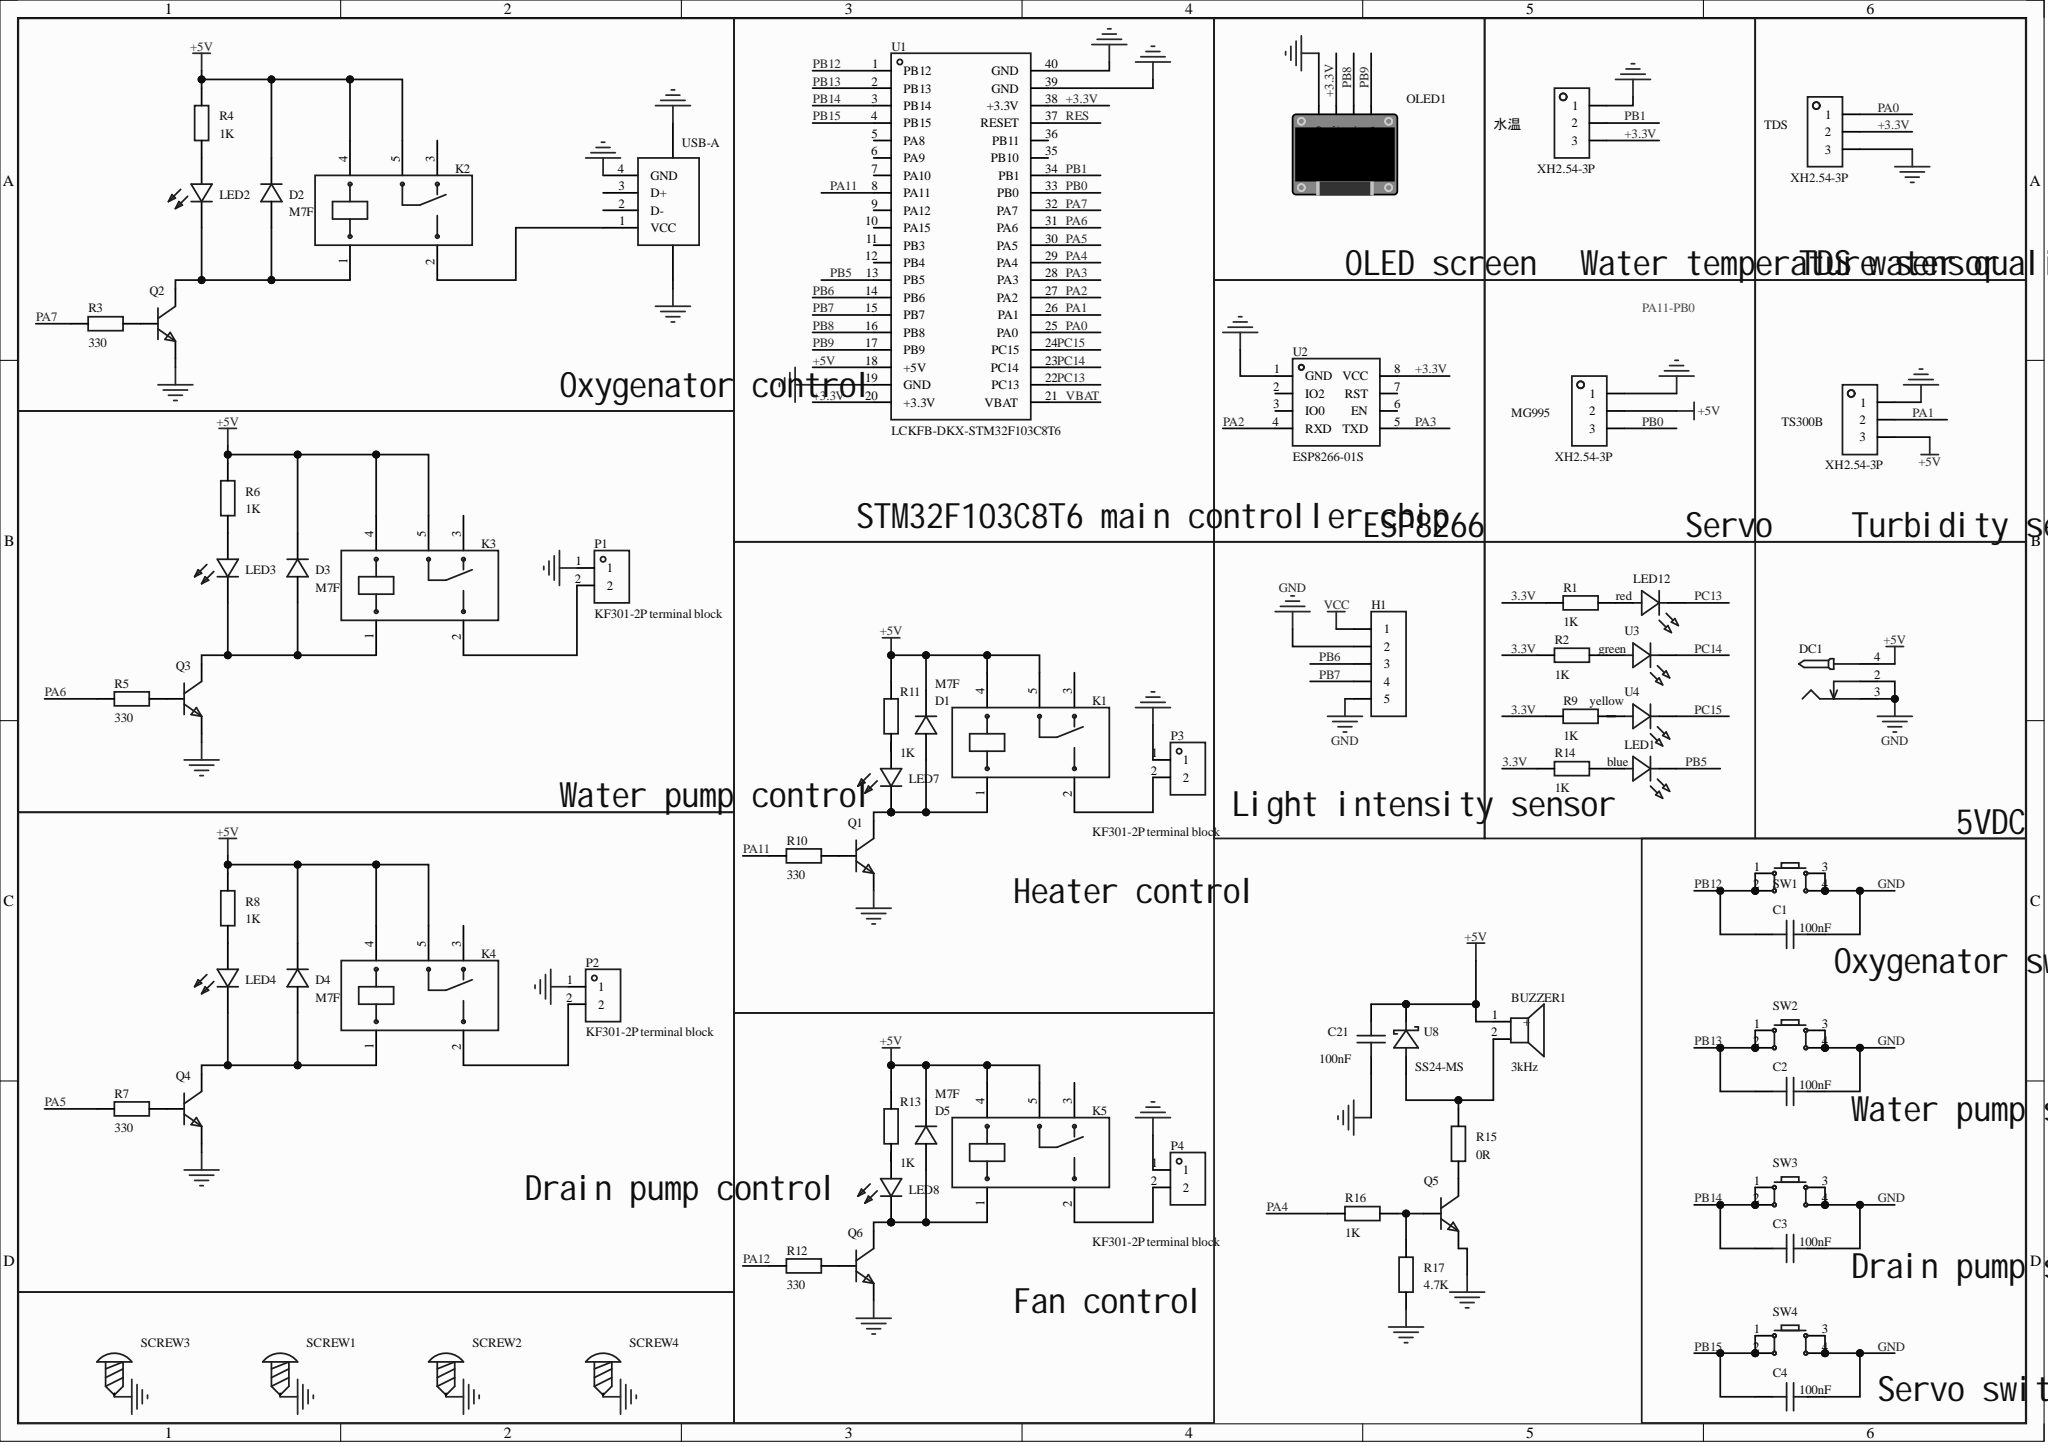Circuit board | Altium Designer | 71 parts | 53 nets
Bill of materials:
Comment,Description,Designator,Footprint,LibRef,Quantity
"3kHz","Drive method: Active (built-in driver circuit); Construction type: Electromagnetic; Rated voltage: -; Frequency: 3kHz; Sound pressure (SPL): 85dB;","BUZZER1","BUZ-TH_BD9.6-P5.00-D0.7-FD","HNB09A05","1"
"100nF","Capacitance: 100nF; Tolerance: ±10%; Rated voltage: 6.3V; Dielectric (temp. coefficient): X7R;, [NoValue]","C1, C2, C3, C4, C21","C0603","CC0603KRX7R5BB104, CAP_0603","5"
"M7F","Forward voltage drop (Vf): 1.1V@1A; DC reverse withstand voltage (Vr): 1kV; Rectifier current: 1A;","D1, D2, D3, D4, D5","SMAF_L3.5-W2.6-LS4.7-RD","M7F_C22368801","5"
"","","DC1","DC-2.0","DC-005_2.0","1"
"","","H1","HDR-TH_5P-P2.54-V-F","HDR-F_2.54_1x5P","1"
"SRD-DC5V-SL-C","Contact form: -;","K1, K2, K3, K4, K5","RELAY-TH_SRD-DCXXV-SL-C","SRD-DC5V-SL-C","5"
"blue","Lamp holder type: 5mm round lamp holder; Emitting color: Blue; Forward voltage drop (Vf): 3.4V; Power: 70mW; Forward current: 20mA; Wavelength: 460nm~470nm; Diode configuration: -; Lens color: Blue lens; Color temperature: -; Luminous intensity: 3cd; Viewing angle: 25°; Tape and reel: -; Operating temperature: -20℃~+85℃;","LED1","LED-TH_BD5.9-P2.54-RD_BLUE","XL-502UBD","1"
"MS-PTV1608NWAF-B02","","LED2, LED3, LED4, LED7, LED8","LED0603-RD","MS-PTV1608NWAF-B02","5"
"red","Lamp holder type: 5mm round lamp holder; Emitting color: Red; Forward voltage drop (Vf): 2.4V; Power: 70mW; Forward current: 20mA; Wavelength: 615nm~625nm; Diode configuration: -; Lens color: Red lens; Color temperature: -; Luminous intensity: 300mcd; Viewing angle: 35°; Tape and reel: -; Operating temperature: -25℃~+85℃;","LED12","LED-TH_BD5.9-P2.54-RD_RED","XL-502SURD","1"
"","","MG995, TDS, TS300B, 水温","XH2.54-3P","弯针座3P","4"
"","","OLED1","0.96OLED_4P","0.96OLED模块_4P","1"
"KF301-2P terminal block","","P1, P2, P3, P4","CONN-TH_XY301V-A-5.0-2P","KF301-2P接线端子","4"
"","","Q1, Q2, Q3, Q4, Q5, Q6","S8050_SOT-23","S8050_SOT_NPN","6"
"1K","","R1, R2, R4, R6, R8, R9, R11, R13, R14, R16","R0603","Res_0603","10"
"330","","R3, R5, R7, R10, R12","R0603","Res_0603","5"
"0R","","R15","R0603","Res_0603","1"
"4.7K","","R17","R0603","Res_0603","1"
"","","SCREW1, SCREW2, SCREW3, SCREW4","M3螺丝","M3螺丝","4"
"","","SW1, SW2, SW3, SW4","SW-SMD_4P-L6.0-W6.0-P4.50-LS9.0-2","Key_SMD_6x6x6.5","4"
"LCKFB-DKX-STM32F103C8T6","","U1","CONN-TH_L53.3-W22.9_STM32F103C8T6-CARD","LCKFB-DKX-STM32F103C8T6","1"
"ESP8266-01S","","U2","WIFIM-TH_ESP8266-01S","ESP8266-01S","1"
"green","Lamp holder type: 5mm round lamp holder; Emitting color: Emerald green; Forward voltage drop (Vf): 3V; Power: 70mW; Forward current: 20mA; Wavelength: 520nm~530nm; Diode configuration: -; Lens color: Green lens; Color temperature: -; Luminous intensity: 12cd; Viewing angle: 25°; Tape and reel: -; Operating temperature: -25℃~+85℃;","U3","LED-TH_BD5.9-P2.54-RD_GREEN","XL-502UGD","1"
"yellow","Lamp holder type: 5mm round lamp holder; Emitting color: Yellow; Forward voltage drop (Vf): 2.2V; Power: 50mW; Forward current: 20mA; Wavelength: 585nm~595nm; Diode configuration: -; Lens color: Yellow lens; Color temperature: -; Luminous intensity: 1cd; Viewing angle: 25°; Tape and reel: -; Operating temperature: -20℃~+85℃;","U4","LED-TH_BD5.9-P2.54-RD_YELLOW","XL-502UYD","1"
"SS24-MS","Diode configuration: -; Forward voltage drop (Vf): 550mV@2A; DC reverse withstand voltage (Vr): 40V; Rectifier current: 2A;","U8","SMA_L4.3-W2.6-LS5.1-RD","SS24-MS","1"
"USB-AF","","USB-A","USB-A-TH_USB-302-T","USB-AF","1"
Netlist (Protel format):
[
BUZZER1
BUZ-TH_BD9.6-P5.00-D0.7-FD
3kHz



]
[
C1
C0603
100nF



]
[
C2
C0603
100nF



]
[
C3
C0603
100nF



]
[
C4
C0603
100nF



]
[
C21
C0603
100nF



]
[
D1
SMAF_L3.5-W2.6-LS4.7-RD
M7F



]
[
D2
SMAF_L3.5-W2.6-LS4.7-RD
M7F



]
[
D3
SMAF_L3.5-W2.6-LS4.7-RD
M7F



]
[
D4
SMAF_L3.5-W2.6-LS4.7-RD
M7F



]
[
D5
SMAF_L3.5-W2.6-LS4.7-RD
M7F



]
[
DC1
DC-2.0




]
[
H1
HDR-TH_5P-P2.54-V-F




]
[
K1
RELAY-TH_SRD-DCXXV-SL-C
SRD-DC5V-SL-C



]
[
K2
RELAY-TH_SRD-DCXXV-SL-C
SRD-DC5V-SL-C



]
[
K3
RELAY-TH_SRD-DCXXV-SL-C
SRD-DC5V-SL-C



]
[
K4
RELAY-TH_SRD-DCXXV-SL-C
SRD-DC5V-SL-C



]
[
K5
RELAY-TH_SRD-DCXXV-SL-C
SRD-DC5V-SL-C



]
[
LED1
LED-TH_BD5.9-P2.54-RD_BLUE
blue



]
[
LED2
LED0603-RD
MS-PTV1608NWAF-B02



]
[
LED3
LED0603-RD
MS-PTV1608NWAF-B02



]
[
LED4
LED0603-RD
MS-PTV1608NWAF-B02



]
[
LED7
LED0603-RD
MS-PTV1608NWAF-B02



]
[
LED8
LED0603-RD
MS-PTV1608NWAF-B02



]
[
LED12
LED-TH_BD5.9-P2.54-RD_RED
red



]
[
MG995
XH2.54-3P




]
[
OLED1
0.96OLED_4P




]
[
P1
CONN-TH_XY301V-A-5.0-2P
KF301-2P terminal block



]
[
P2
CONN-TH_XY301V-A-5.0-2P
KF301-2P terminal block



]
[
P3
CONN-TH_XY301V-A-5.0-2P
KF301-2P terminal block



]
[
P4
CONN-TH_XY301V-A-5.0-2P
KF301-2P terminal block



]
[
Q1
S8050_SOT-23




]
[
Q2
S8050_SOT-23




]
[
Q3
S8050_SOT-23




]
[
Q4
S8050_SOT-23




]
[
Q5
S8050_SOT-23




]
[
Q6
S8050_SOT-23




]
[
R1
R0603
1K



]
[
R2
R0603
1K



]
[
R3
R0603
330



]
[
R4
R0603
1K



]
[
R5
R0603
330



]
[
R6
R0603
1K



]
[
R7
R0603
330



]
[
R8
R0603
1K



]
[
R9
R0603
1K



]
[
R10
R0603
330



]
[
R11
R0603
1K



]
[
R12
R0603
330



]
[
R13
R0603
1K



]
[
R14
R0603
1K



]
[
R15
R0603
0R



]
[
R16
R0603
1K



]
[
R17
R0603
4.7K



]
[
SCREW1
M3螺丝




]
[
SCREW2
M3螺丝




]
[
SCREW3
M3螺丝




]
[
SCREW4
M3螺丝




]
[
SW1
SW-SMD_4P-L6.0-W6.0-P4.50-LS9.0-2




]
[
SW2
SW-SMD_4P-L6.0-W6.0-P4.50-LS9.0-2




]
[
SW3
SW-SMD_4P-L6.0-W6.0-P4.50-LS9.0-2




]
[
SW4
SW-SMD_4P-L6.0-W6.0-P4.50-LS9.0-2




]
[
TDS
XH2.54-3P




]
[
TS300B
XH2.54-3P




]
[
U1
CONN-TH_L53.3-W22.9_STM32F103C8T6-CARD
LCKFB-DKX-STM32F103C8T6



]
[
U2
WIFIM-TH_ESP8266-01S
ESP8266-01S



]
[
U3
LED-TH_BD5.9-P2.54-RD_GREEN
green



]
[
U4
LED-TH_BD5.9-P2.54-RD_YELLOW
yellow



]
[
U8
SMA_L4.3-W2.6-LS5.1-RD
SS24-MS



]
[
USB-A
USB-A-TH_USB-302-T
USB-AF



]
[
水温
XH2.54-3P




]
(
PC15
U1-24
U4-1
)
(
PC14
U1-23
U3-1
)
(
PC13
LED12-1
U1-22
)
(
PB15
C4-1
SW4-1
SW4-2
U1-4
)
(
PB14
C3-1
SW3-1
SW3-2
U1-3
)
(
PB13
C2-1
SW2-1
SW2-2
U1-2
)
(
PB12
C1-1
SW1-1
SW1-2
U1-1
)
(
PB9
OLED1-4
U1-17
)
(
PB8
OLED1-3
U1-16
)
(
PB7
H1-4
U1-15
)
(
PB6
H1-3
U1-14
)
(
PB5
LED1-1
U1-13
)
(
PB1
U1-34
水温-2
)
(
PB0
MG995-3
U1-33
)
(
PA11
R10-2
U1-8
)
(
PA7
R3-2
U1-32
)
(
PA6
R5-2
U1-31
)
(
PA5
R7-2
U1-30
)
(
PA4
R16-2
U1-29
)
(
PA3
U1-28
U2-5
)
(
PA2
U1-27
U2-4
)
(
PA1
TS300B-2
U1-26
)
(
PA0
TDS-1
U1-25
)
(
NetR9_2
R9-2
U4-2
)
(
NetR2_2
R2-2
U3-2
)
(
NetQ6_1
Q6-1
R12-1
)
(
NetQ5_3
Q5-3
R15-1
)
(
NetQ5_1
Q5-1
R16-1
R17-1
)
(
NetQ4_1
Q4-1
R7-1
)
(
NetQ3_1
Q3-1
R5-1
)
(
NetQ2_1
Q2-1
R3-1
)
(
NetQ1_1
Q1-1
R10-1
)
(
NetLED12_2
LED12-2
R1-2
)
(
NetLED8_2
LED8-2
R13-1
)
(
NetLED7_2
LED7-2
R11-1
)
(
NetLED4_2
LED4-2
R8-1
)
(
NetLED3_2
LED3-2
R6-1
)
(
NetLED2_2
LED2-2
R4-1
)
(
NetLED1_2
LED1-2
R14-2
)
(
NetK5_2
K5-2
P4-2
)
(
NetK4_2
K4-2
P2-2
)
(
NetK3_2
K3-2
P1-2
)
(
NetK2_2
K2-2
USB-A-1
)
(
NetK1_2
K1-2
P3-2
)
(
NetD5_2
D5-2
K5-1
LED8-1
Q6-3
)
(
NetD4_2
D4-2
K4-1
LED4-1
Q4-3
)
(
NetD3_2
D3-2
K3-1
LED3-1
Q3-3
)
(
NetD2_2
D2-2
K2-1
LED2-1
Q2-3
)
(
NetD1_2
D1-2
K1-1
LED7-1
Q1-3
)
(
NetBUZZER1_2
BUZZER1-2
R15-2
U8-2
)
(
GND
C1-2
C2-2
C3-2
C4-2
C21-1
DC1-2
DC1-3
H1-2
H1-5
MG995-1
OLED1-1
P1-1
P2-1
P3-1
P4-1
Q1-2
Q2-2
Q3-2
Q4-2
Q5-2
Q6-2
R17-2
SCREW1-1
SCREW2-1
SCREW3-1
SCREW4-1
SW1-3
SW1-4
SW2-3
SW2-4
SW3-3
SW3-4
SW4-3
SW4-4
TDS-3
TS300B-1
U1-19
U1-39
U1-40
U2-1
USB-A-4
USB-A-5
USB-A-6
水温-1
)
(
+5V
BUZZER1-1
C21-2
D1-1
D2-1
D3-1
D4-1
D5-1
DC1-4
K1-4
K1-5
K2-4
K2-5
K3-4
K3-5
K4-4
K4-5
K5-4
K5-5
MG995-2
R4-2
R6-2
R8-2
R11-2
R13-2
TS300B-3
U1-18
U8-1
)
(
3.3V
H1-1
OLED1-2
R1-1
R2-1
R9-1
R14-1
TDS-2
U1-20
U1-38
U2-8
水温-3
)